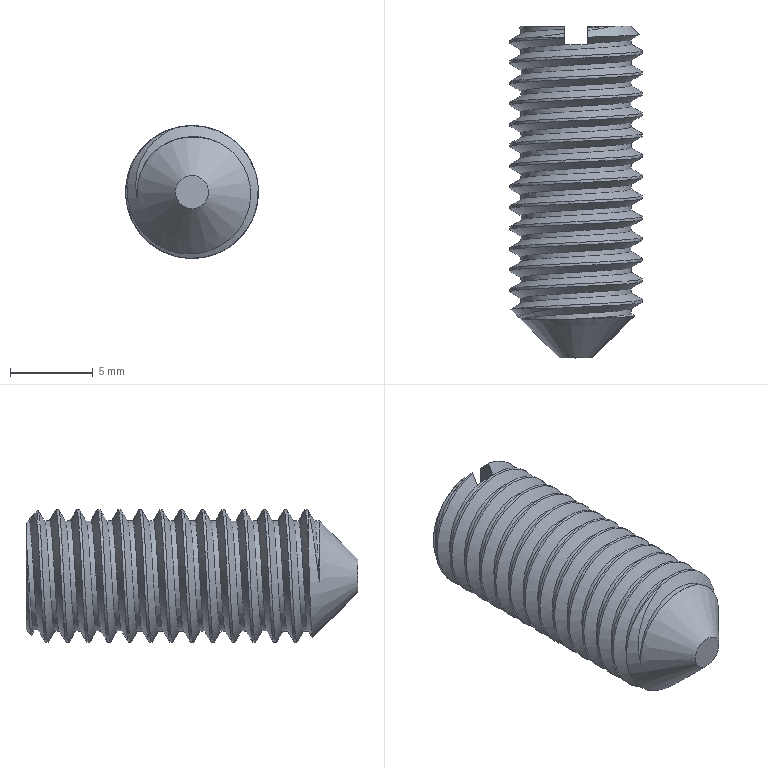Part | NX | features DATUM_CSYS 3, SKETCH 2, CHAMFER 1, EXTRUDE 1, SWP104 1, THREADS 1 | 1 solid | 22 faces | box 8 x 20 x 8 mm | volume 753.077 mm3 | plane 7 | spline 6 | cylinder 5 | cone 4 | commonest cylinder face diameters 6.647 x3 1.2 x1 8 x1